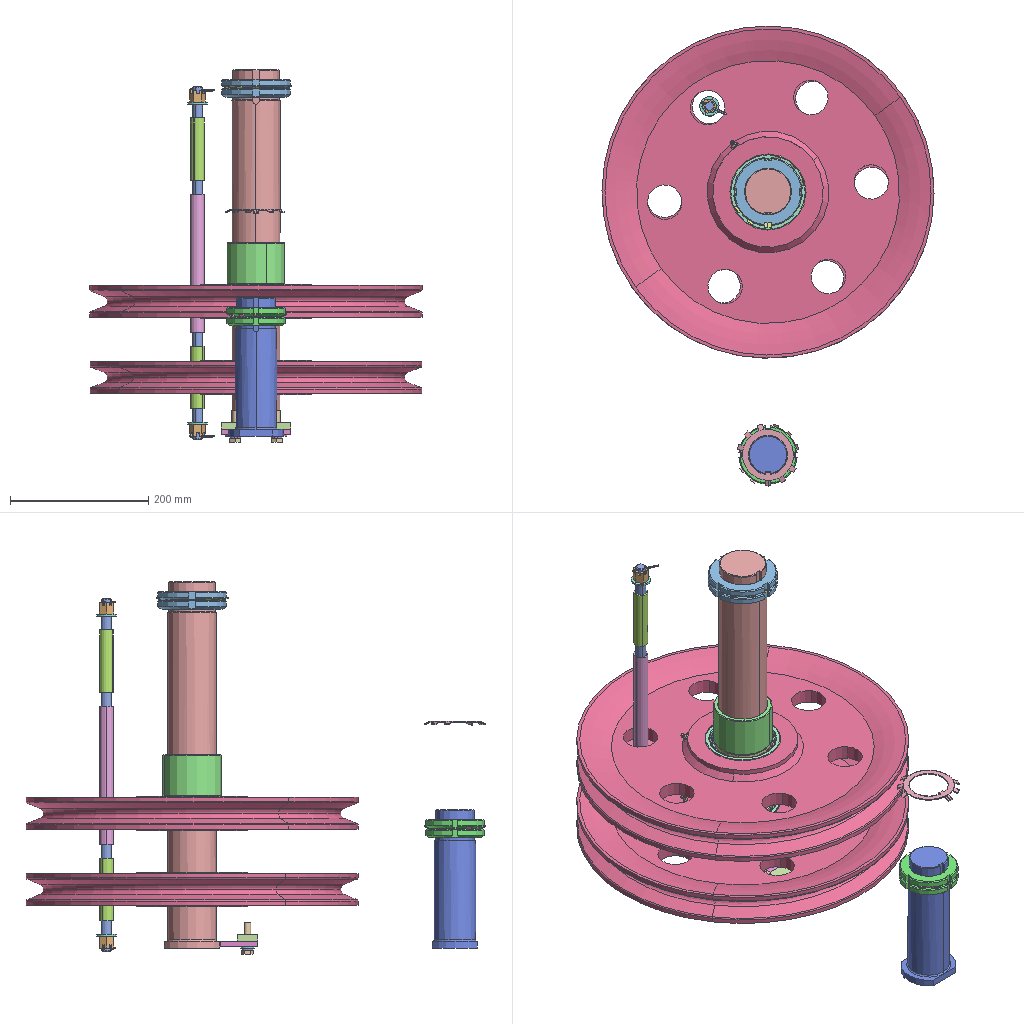Assembly | SolidWorks | 24 different items | 40 placed | box 480 x 665 x 539 mm
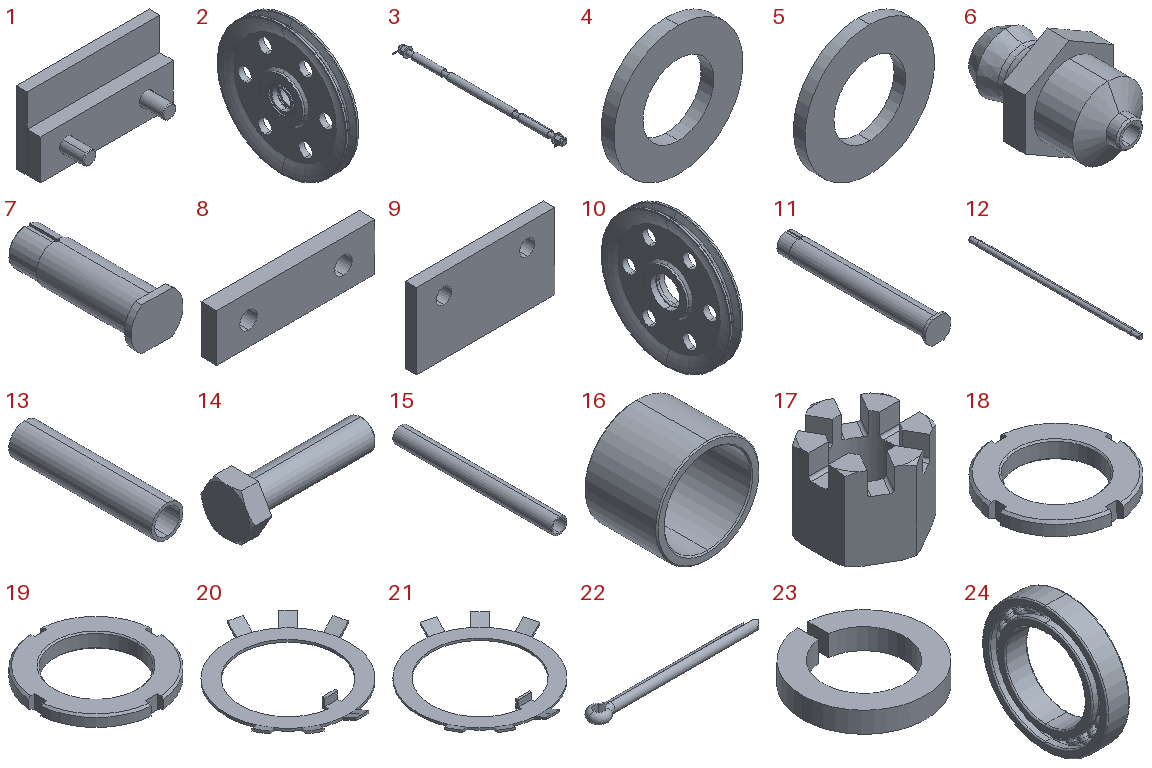Parts list (item | name | quantity | parent item | size | volume | features):
1 | (subassembly) | x1 | - | 100 x 46.4 x 54.5 mm | 80698 mm3 | features ReferencePattern 3, CompositeCurve 1, MirrorCompFeat 1
2 | (subassembly) | x2 | - | 50 x 480 x 480 mm | 4092545 mm3 | features CompositeCurve 1
3 | (subassembly) | x1 | - | 41.5 x 510 x 28 mm | 141219 mm3 | features CompositeCurve 2
4 | - | x2 | in 1 | 20 x 2 x 20 mm | 438.252 mm3 | features Revolution 1
5 | - | x2 | in 3 | 28 x 2.5 x 28 mm | 1068 mm3 | features Revolution 1
6 | - | x2 | in 2 | 10 x 16 x 11.547 mm | 627.343 mm3 | features Boss 1, Chamfer 1, Revolution 1
7 | - | x1 | - | 80 x 200 x 65 mm | 564846 mm3 | features Fillet 2, ICE 2, Chamfer 1, Revolution 1
8 | - | x1 | in 1 | 100 x 10 x 30 mm | 28099 mm3 | features Extrusion 1, HoleWzd 1
9 | - | x1 | in 1 | 100 x 8 x 54.5 mm | 42079 mm3 | features Extrusion 1, HoleWzd 1
10 | - | x2 | in 2 | 50 x 480 x 480 mm | 3922963 mm3 | features ICE 2, Chamfer 1, Fillet 1, MirrorPattern 1, RevCut 1, Revolution 1
11 | - | x1 | - | 90 x 530 x 80 mm | 2050473 mm3 | features Fillet 2, ICE 2, Chamfer 1, Revolution 1
12 | - | x1 | in 3 | 15 x 510 x 15 mm | 88747 mm3 | features Chamfer 1, ICE 1, Revolution 1
13 | - | x2 | in 3 | 20 x 90 x 20 mm | 10179 mm3 | features WeldMemberFeat 1, WeldmentFeature 1
14 | - | x2 | in 1 | 46.4 x 18.475 x 16 mm | 4560 mm3 | features Chamfer 2, RevCut 2, Revolution 2, Extrusion 1, ICE 1
15 | - | x1 | in 3 | 20 x 200 x 20 mm | 22619 mm3 | features WeldMemberFeat 1, WeldmentFeature 1
16 | - | x1 | - | 85 x 60 x 85 mm | 102428 mm3 | features Chamfer 1, Extrusion 1
17 | - | x2 | in 3 | 19.728 x 22.78 x 17.8 mm | 3522 mm3 | features Cut 3, Chamfer 1, CirPattern 1, Extrusion 1
18 | - | x2 | - | 84.623 x 84.623 x 12 mm | 36703 mm3 | features Chamfer 3, CirPattern 1, Cut 1, Extrusion 1
19 | - | x2 | - | 99.499 x 99.499 x 12 mm | 47793 mm3 | features Chamfer 3, CirPattern 1, Cut 1, Extrusion 1
20 | - | x2 | - | 85.057 x 89.139 x 6 mm | 3268 mm3 | features Boss 1, Cut 1, Revolution 1
21 | - | x1 | - | 99.417 x 104.021 x 6 mm | 4358 mm3 | features Boss 1, Cut 1, Revolution 1
22 | - | x2 | in 3 | 39.5 x 4.6 x 2.3 mm | 158.041 mm3 | features ICE 1, Sweep 1
23 | - | x2 | in 1 | 15.372 x 15.344 x 2.6 mm | 261.313 mm3 | features Extrusion 1
24 | - | x4 | in 2 | 20 x 110 x 110 mm | 84477 mm3 | features Revolution 5, CirPattern 2, RefAxis 1, RevCut 1
Mates (type | each side: item.copy, entity, surface, feature):
In the top assembly
Concentric | 11.1 face cylinder Revolve1 | 16.1 face cylinder Boss-Extrude1
Concentric | 19.1 face cylinder Base-Extrude | 19.2 face cylinder Base-Extrude
Coincident | 19.1 face plane CirPattern1 | 19.2 face plane CirPattern1
Concentric | 19.1 face cylinder Base-Extrude | 21.1 face cylinder Cut-Extrude2
Coincident | 21.1 face plane Base-Revolve | 19.2 face plane Base-Extrude
Parallel | 21.1 face plane Cut-Extrude2 | 19.2 face plane Cut-Extrude1
Coincident | 19.1 face plane Base-Extrude | 21.1 face plane Base-Revolve
Concentric | 11.1 face cylinder Revolve1 | 19.2 face cylinder Base-Extrude
Concentric | 11.1 face cylinder Revolve1 | 24.1 face cylinder Revolve1
Concentric | 11.1 face cylinder Revolve1 | 24.2 face cylinder Revolve1
Coincident | 16.1 face plane Boss-Extrude1 | 24.2 face plane Revolve1
Concentric | 18.1 face cylinder Base-Extrude | 7.1 face cylinder Revolve1
Concentric | 7.1 face cylinder Revolve1 | 18.2 face cylinder Base-Extrude
Concentric | 20.1 face cylinder Cut-Extrude2 | 18.2 face cylinder Base-Extrude
Coincident | 18.1 face plane Cut-Extrude1 | 18.2 face plane Cut-Extrude1
Coincident | 18.1 face plane Base-Extrude | 20.1 face plane Base-Revolve
Parallel | 20.1 face plane Cut-Extrude2 | 7.1 face plane Cut-Extrude2
Coincident | 20.1 face plane Base-Revolve | 18.2 face plane Base-Extrude
Coincident | 18.1 face plane CirPattern1 | 7.1 face plane Cut-Extrude2
Concentric | 15.1 face cylinder GB/T 6728-2002 round tube 20 × 2(1) | 10.1 face cylinder Cut-Extrude1
In subassembly 2
Concentric | 10.2 face cylinder Cut-Extrude1 | 24.3 face cylinder Revolve1
Concentric | 10.2 face cylinder Mirror1 | 24.4 edge
Coincident | 10.2 face plane Cut-Extrude2 | 24.4 face plane Revolve1
Coincident | 10.2 face plane Mirror1 | 24.3 face plane Revolve1
Concentric | 10.2 face cylinder Cut-Revolve1 | 6.1 face cylinder Revolve2
Coincident | 10.2 edge | 6.1 face plane Revolve2
In subassembly 3
Coordinate | 12.1 select_type:25 | 3.1 select_type:11
Concentric | 17.1 face cylinder Base-Extrude | 5.1 face cylinder Base-Revolve
Coincident | 17.1 face plane Base-Extrude | 5.1 face plane Base-Revolve
Concentric | 12.1 face cylinder Revolve1 | 5.1 face cylinder Base-Revolve
Coincident | 12.1 face plane Revolve1 | 5.1 face plane Base-Revolve
Concentric | 5.2 face cylinder Base-Revolve | 17.2 face cylinder Base-Extrude
Coincident | 5.2 face plane Base-Revolve | 17.2 face plane Base-Extrude
Parallel | 17.1 face plane Base-Extrude | 17.2 face plane Base-Extrude
Concentric | 12.1 face cylinder Revolve1 | 5.2 face cylinder Base-Revolve
Coincident | 12.1 face plane Revolve1 | 5.2 face plane Base-Revolve
Concentric | 12.1 face cylinder Revolve1 | 15.2 face cylinder GB/T 6728-2002 round tube 20 × 2(1)
Concentric | 12.1 face cylinder Revolve1 | 13.1 face cylinder GB/T 6728-2002 round tube 20 × 2(1)
Concentric | 12.1 face cylinder Revolve1 | 13.2 face cylinder GB/T 6728-2002 round tube 20 × 2(1)
DistanceDim | 13.1 face plane GB/T 6728-2002 round tube 20 × 2(1) | 5.1 face plane Base-Revolve
DistanceDim | 15.2 face plane GB/T 6728-2002 round tube 20 × 2(1) | 13.1 face plane GB/T 6728-2002 round tube 20 × 2(1)
DistanceDim | 15.2 face plane GB/T 6728-2002 round tube 20 × 2(1) | 13.2 face plane GB/T 6728-2002 round tube 20 × 2(1)
Parallel | 17.1 face plane Base-Extrude | 3.1 plane
Concentric | 12.1 face cylinder Cut-Extrude1 | 22.1 face cylinder Sweep2
Parallel | 5.1 face plane Base-Revolve | 22.1 face plane Sweep2
Tangent | 12.1 face cylinder Revolve1 | 22.1 edge
Concentric | 12.1 face cylinder Cut-Extrude1 | 22.2 face cylinder Sweep2
Tangent | 12.1 face cylinder Revolve1 | 22.2 edge
Parallel | 5.2 face plane Base-Revolve | 22.2 face plane Sweep2
In subassembly 1
Coordinate | 8.1 select_type:25 | 1.1 select_type:11
Concentric | 8.1 face cylinder Ø11.0 (11) Diameter Hole1 | 9.1 face cylinder Ø11.0 (11) Diameter Hole1
Coincident | 8.1 face plane Boss-Extrude1 | 9.1 face plane Boss-Extrude1 | 2 times
Concentric | 14.1 face cylinder Revolve1 | 23.1 face cylinder Extrude1
Concentric | 14.1 face cylinder Revolve1 | 4.1 face cylinder Base-Revolve
Concentric | 9.1 face cylinder Ø11.0 (11) Diameter Hole1 | 14.1 face cylinder Revolve1
Coincident | 4.1 face plane Base-Revolve | 23.1 face plane Extrude1
Coincident | 14.1 face plane Boss-Extrude1 | 23.1 face plane Extrude1
Coincident | 9.1 face plane Boss-Extrude1 | 4.1 face plane Base-Revolve
Parallel | 9.1 face plane Boss-Extrude1 | 14.1 face plane Boss-Extrude1